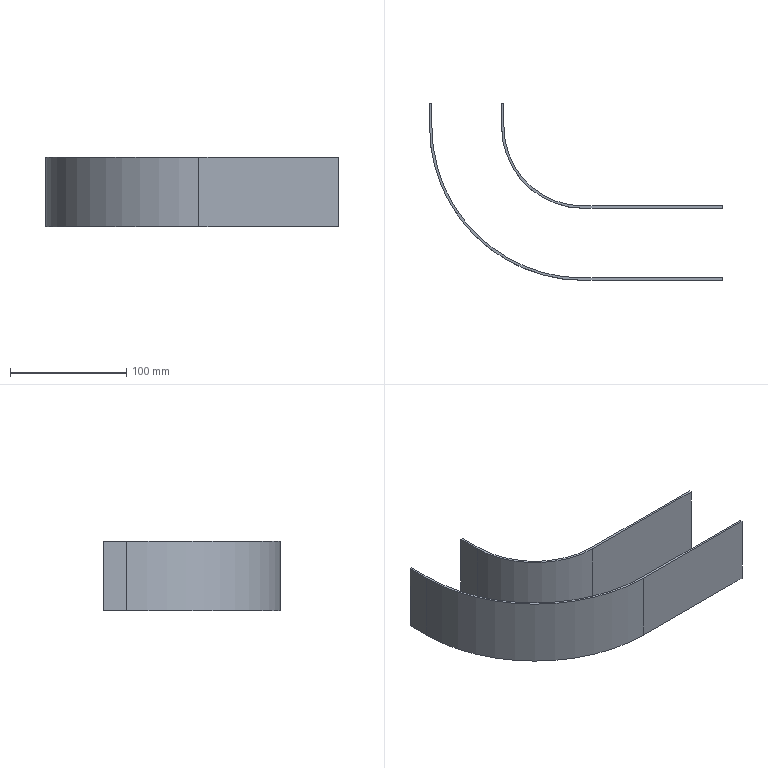Part | STEP file | 2 solids | 20 faces | box 252 x 152 x 60 mm | volume 71299 mm3 | plane 16 | cylinder 4 | commonest cylinder face diameters 136 x1 140 x1 260 x1 264 x1
STEP:
#1=CARTESIAN_POINT('',(0.,0.,0.));
#2=DIRECTION('',(0.,0.,1.));
#3=DIRECTION('',(1.,0.,0.));
#4=AXIS2_PLACEMENT_3D('',#1,#2,#3);
#5=CARTESIAN_POINT('',(100.,-32.,60.));
#6=VERTEX_POINT('',#5);
#7=CARTESIAN_POINT('',(-32.,100.,60.));
#8=VERTEX_POINT('',#7);
#9=CARTESIAN_POINT('',(100.,100.,60.));
#10=DIRECTION('',(0.,0.,-1.));
#11=DIRECTION('',(1.,0.,0.));
#12=AXIS2_PLACEMENT_3D('',#9,#10,#11);
#13=CIRCLE('',#12,132.);
#14=CARTESIAN_POINT('',(100.,100.,60.));
#15=DIRECTION('',(0.,0.,1.));
#16=DIRECTION('',(1.,0.,0.));
#17=AXIS2_PLACEMENT_3D('',#14,#15,#16);
#18=CYLINDRICAL_SURFACE('',#17,132.);
#19=CARTESIAN_POINT('',(6.283,0.));
#20=DIRECTION('',(-1.,0.));
#21=VECTOR('',#20,1.);
#22=LINE('',#19,#21);
#23=(GEOMETRIC_REPRESENTATION_CONTEXT(2)PARAMETRIC_REPRESENTATION_CONTEXT()REPRESENTATION_CONTEXT('',''));
#24=DEFINITIONAL_REPRESENTATION('',(#22),#23);
#25=PCURVE('',#18,#24);
#26=CARTESIAN_POINT('',(100.,100.,60.));
#27=DIRECTION('',(0.,0.,1.));
#28=DIRECTION('',(1.,0.,0.));
#29=AXIS2_PLACEMENT_3D('',#26,#27,#28);
#30=PLANE('',#29);
#31=CARTESIAN_POINT('',(132.,0.));
#32=CARTESIAN_POINT('',(132.,-228.631));
#33=CARTESIAN_POINT('',(-66.,-114.315));
#34=CARTESIAN_POINT('',(-264.,0.));
#35=CARTESIAN_POINT('',(-66.,114.315));
#36=CARTESIAN_POINT('',(132.,228.631));
#37=CARTESIAN_POINT('',(132.,0.));
#38=(BOUNDED_CURVE()B_SPLINE_CURVE(2,(#31,#32,#33,#34,#35,#36,#37),.UNSPECIFIED.,.T.,.F.)B_SPLINE_CURVE_WITH_KNOTS((1,2,2,2,2,1),(-2.094,0.,2.094,4.189,6.283,8.378),.UNSPECIFIED.)CURVE()GEOMETRIC_REPRESENTATION_ITEM()RATIONAL_B_SPLINE_CURVE((1.,0.5,1.,0.5,1.,0.5,1.))REPRESENTATION_ITEM(''));
#39=(GEOMETRIC_REPRESENTATION_CONTEXT(2)PARAMETRIC_REPRESENTATION_CONTEXT()REPRESENTATION_CONTEXT('',''));
#40=DEFINITIONAL_REPRESENTATION('',(#38),#39);
#41=PCURVE('',#30,#40);
#42=SURFACE_CURVE('',#13,(#25,#41),.PCURVE_S1.);
#43=EDGE_CURVE('',#6,#8,#42,.T.);
#44=ORIENTED_EDGE('',*,*,#43,.T.);
#45=CARTESIAN_POINT('',(-32.,100.,0.));
#46=VERTEX_POINT('',#45);
#47=CARTESIAN_POINT('',(-32.,100.,60.));
#48=DIRECTION('',(0.,0.,-1.));
#49=VECTOR('',#48,1.);
#50=LINE('',#47,#49);
#51=CARTESIAN_POINT('',(3.142,0.));
#52=DIRECTION('',(0.,-1.));
#53=VECTOR('',#52,1.);
#54=LINE('',#51,#53);
#55=(GEOMETRIC_REPRESENTATION_CONTEXT(2)PARAMETRIC_REPRESENTATION_CONTEXT()REPRESENTATION_CONTEXT('',''));
#56=DEFINITIONAL_REPRESENTATION('',(#54),#55);
#57=PCURVE('',#18,#56);
#58=CARTESIAN_POINT('',(-32.,100.,60.));
#59=DIRECTION('',(-1.,0.,0.));
#60=DIRECTION('',(0.,0.,1.));
#61=AXIS2_PLACEMENT_3D('',#58,#59,#60);
#62=PLANE('',#61);
#63=CARTESIAN_POINT('',(0.,0.));
#64=DIRECTION('',(-1.,0.));
#65=VECTOR('',#64,1.);
#66=LINE('',#63,#65);
#67=(GEOMETRIC_REPRESENTATION_CONTEXT(2)PARAMETRIC_REPRESENTATION_CONTEXT()REPRESENTATION_CONTEXT('',''));
#68=DEFINITIONAL_REPRESENTATION('',(#66),#67);
#69=PCURVE('',#62,#68);
#70=SURFACE_CURVE('',#50,(#57,#69),.PCURVE_S1.);
#71=EDGE_CURVE('',#8,#46,#70,.T.);
#72=ORIENTED_EDGE('',*,*,#71,.T.);
#73=CARTESIAN_POINT('',(100.,-32.,0.));
#74=VERTEX_POINT('',#73);
#75=CARTESIAN_POINT('',(100.,100.,0.));
#76=DIRECTION('',(0.,0.,1.));
#77=DIRECTION('',(1.,0.,0.));
#78=AXIS2_PLACEMENT_3D('',#75,#76,#77);
#79=CIRCLE('',#78,132.);
#80=CARTESIAN_POINT('',(0.,-60.));
#81=DIRECTION('',(1.,0.));
#82=VECTOR('',#81,1.);
#83=LINE('',#80,#82);
#84=(GEOMETRIC_REPRESENTATION_CONTEXT(2)PARAMETRIC_REPRESENTATION_CONTEXT()REPRESENTATION_CONTEXT('',''));
#85=DEFINITIONAL_REPRESENTATION('',(#83),#84);
#86=PCURVE('',#18,#85);
#87=CARTESIAN_POINT('',(100.,100.,0.));
#88=DIRECTION('',(0.,0.,1.));
#89=DIRECTION('',(1.,0.,0.));
#90=AXIS2_PLACEMENT_3D('',#87,#88,#89);
#91=PLANE('',#90);
#92=CARTESIAN_POINT('',(0.,0.));
#93=DIRECTION('',(1.,0.));
#94=AXIS2_PLACEMENT_2D('',#92,#93);
#95=CIRCLE('',#94,132.);
#96=(GEOMETRIC_REPRESENTATION_CONTEXT(2)PARAMETRIC_REPRESENTATION_CONTEXT()REPRESENTATION_CONTEXT('',''));
#97=DEFINITIONAL_REPRESENTATION('',(#95),#96);
#98=PCURVE('',#91,#97);
#99=SURFACE_CURVE('',#79,(#86,#98),.PCURVE_S1.);
#100=EDGE_CURVE('',#46,#74,#99,.T.);
#101=ORIENTED_EDGE('',*,*,#100,.T.);
#102=CARTESIAN_POINT('',(100.,-32.,60.));
#103=DIRECTION('',(0.,0.,1.));
#104=VECTOR('',#103,1.);
#105=LINE('',#102,#104);
#106=CARTESIAN_POINT('',(4.712,0.));
#107=DIRECTION('',(0.,1.));
#108=VECTOR('',#107,1.);
#109=LINE('',#106,#108);
#110=(GEOMETRIC_REPRESENTATION_CONTEXT(2)PARAMETRIC_REPRESENTATION_CONTEXT()REPRESENTATION_CONTEXT('',''));
#111=DEFINITIONAL_REPRESENTATION('',(#109),#110);
#112=PCURVE('',#18,#111);
#113=CARTESIAN_POINT('',(100.,-32.,60.));
#114=DIRECTION('',(0.,-1.,0.));
#115=DIRECTION('',(0.,0.,-1.));
#116=AXIS2_PLACEMENT_3D('',#113,#114,#115);
#117=PLANE('',#116);
#118=CARTESIAN_POINT('',(0.,0.));
#119=DIRECTION('',(-1.,0.));
#120=VECTOR('',#119,1.);
#121=LINE('',#118,#120);
#122=(GEOMETRIC_REPRESENTATION_CONTEXT(2)PARAMETRIC_REPRESENTATION_CONTEXT()REPRESENTATION_CONTEXT('',''));
#123=DEFINITIONAL_REPRESENTATION('',(#121),#122);
#124=PCURVE('',#117,#123);
#125=SURFACE_CURVE('',#105,(#112,#124),.PCURVE_S1.);
#126=EDGE_CURVE('',#74,#6,#125,.T.);
#127=ORIENTED_EDGE('',*,*,#126,.T.);
#128=EDGE_LOOP('',(#44,#72,#101,#127));
#129=FACE_BOUND('',#128,.T.);
#130=ADVANCED_FACE('',(#129),#18,.T.);
#131=CARTESIAN_POINT('',(-32.,120.,60.));
#132=VERTEX_POINT('',#131);
#133=CARTESIAN_POINT('',(-32.,100.,60.));
#134=DIRECTION('',(0.,1.,0.));
#135=VECTOR('',#134,1.);
#136=LINE('',#133,#135);
#137=CARTESIAN_POINT('',(0.,0.));
#138=DIRECTION('',(0.,1.));
#139=VECTOR('',#138,1.);
#140=LINE('',#137,#139);
#141=(GEOMETRIC_REPRESENTATION_CONTEXT(2)PARAMETRIC_REPRESENTATION_CONTEXT()REPRESENTATION_CONTEXT('',''));
#142=DEFINITIONAL_REPRESENTATION('',(#140),#141);
#143=PCURVE('',#62,#142);
#144=CARTESIAN_POINT('',(-132.,0.));
#145=DIRECTION('',(0.,1.));
#146=VECTOR('',#145,1.);
#147=LINE('',#144,#146);
#148=(GEOMETRIC_REPRESENTATION_CONTEXT(2)PARAMETRIC_REPRESENTATION_CONTEXT()REPRESENTATION_CONTEXT('',''));
#149=DEFINITIONAL_REPRESENTATION('',(#147),#148);
#150=PCURVE('',#30,#149);
#151=SURFACE_CURVE('',#136,(#143,#150),.PCURVE_S1.);
#152=EDGE_CURVE('',#8,#132,#151,.T.);
#153=ORIENTED_EDGE('',*,*,#152,.T.);
#154=CARTESIAN_POINT('',(-32.,120.,0.));
#155=VERTEX_POINT('',#154);
#156=CARTESIAN_POINT('',(-32.,120.,60.));
#157=DIRECTION('',(0.,0.,-1.));
#158=VECTOR('',#157,1.);
#159=LINE('',#156,#158);
#160=CARTESIAN_POINT('',(0.,20.));
#161=DIRECTION('',(-1.,0.));
#162=VECTOR('',#161,1.);
#163=LINE('',#160,#162);
#164=(GEOMETRIC_REPRESENTATION_CONTEXT(2)PARAMETRIC_REPRESENTATION_CONTEXT()REPRESENTATION_CONTEXT('',''));
#165=DEFINITIONAL_REPRESENTATION('',(#163),#164);
#166=PCURVE('',#62,#165);
#167=CARTESIAN_POINT('',(-32.,120.,60.));
#168=DIRECTION('',(0.,1.,0.));
#169=DIRECTION('',(0.,0.,1.));
#170=AXIS2_PLACEMENT_3D('',#167,#168,#169);
#171=PLANE('',#170);
#172=CARTESIAN_POINT('',(0.,0.));
#173=DIRECTION('',(-1.,0.));
#174=VECTOR('',#173,1.);
#175=LINE('',#172,#174);
#176=(GEOMETRIC_REPRESENTATION_CONTEXT(2)PARAMETRIC_REPRESENTATION_CONTEXT()REPRESENTATION_CONTEXT('',''));
#177=DEFINITIONAL_REPRESENTATION('',(#175),#176);
#178=PCURVE('',#171,#177);
#179=SURFACE_CURVE('',#159,(#166,#178),.PCURVE_S1.);
#180=EDGE_CURVE('',#132,#155,#179,.T.);
#181=ORIENTED_EDGE('',*,*,#180,.T.);
#182=CARTESIAN_POINT('',(-32.,100.,0.));
#183=DIRECTION('',(0.,-1.,0.));
#184=VECTOR('',#183,1.);
#185=LINE('',#182,#184);
#186=CARTESIAN_POINT('',(-60.,0.));
#187=DIRECTION('',(0.,-1.));
#188=VECTOR('',#187,1.);
#189=LINE('',#186,#188);
#190=(GEOMETRIC_REPRESENTATION_CONTEXT(2)PARAMETRIC_REPRESENTATION_CONTEXT()REPRESENTATION_CONTEXT('',''));
#191=DEFINITIONAL_REPRESENTATION('',(#189),#190);
#192=PCURVE('',#62,#191);
#193=CARTESIAN_POINT('',(-132.,0.));
#194=DIRECTION('',(0.,-1.));
#195=VECTOR('',#194,1.);
#196=LINE('',#193,#195);
#197=(GEOMETRIC_REPRESENTATION_CONTEXT(2)PARAMETRIC_REPRESENTATION_CONTEXT()REPRESENTATION_CONTEXT('',''));
#198=DEFINITIONAL_REPRESENTATION('',(#196),#197);
#199=PCURVE('',#91,#198);
#200=SURFACE_CURVE('',#185,(#192,#199),.PCURVE_S1.);
#201=EDGE_CURVE('',#155,#46,#200,.T.);
#202=ORIENTED_EDGE('',*,*,#201,.T.);
#203=ORIENTED_EDGE('',*,*,#71,.F.);
#204=EDGE_LOOP('',(#153,#181,#202,#203));
#205=FACE_BOUND('',#204,.T.);
#206=ADVANCED_FACE('',(#205),#62,.T.);
#207=CARTESIAN_POINT('',(220.,-32.,60.));
#208=VERTEX_POINT('',#207);
#209=CARTESIAN_POINT('',(220.,-30.,60.));
#210=VERTEX_POINT('',#209);
#211=CARTESIAN_POINT('',(220.,100.,60.));
#212=DIRECTION('',(0.,1.,0.));
#213=VECTOR('',#212,1.);
#214=LINE('',#211,#213);
#215=CARTESIAN_POINT('',(120.,0.));
#216=DIRECTION('',(0.,1.));
#217=VECTOR('',#216,1.);
#218=LINE('',#215,#217);
#219=(GEOMETRIC_REPRESENTATION_CONTEXT(2)PARAMETRIC_REPRESENTATION_CONTEXT()REPRESENTATION_CONTEXT('',''));
#220=DEFINITIONAL_REPRESENTATION('',(#218),#219);
#221=PCURVE('',#30,#220);
#222=CARTESIAN_POINT('',(220.,32.,60.));
#223=DIRECTION('',(1.,0.,0.));
#224=DIRECTION('',(0.,0.,-1.));
#225=AXIS2_PLACEMENT_3D('',#222,#223,#224);
#226=PLANE('',#225);
#227=CARTESIAN_POINT('',(0.,68.));
#228=DIRECTION('',(0.,1.));
#229=VECTOR('',#228,1.);
#230=LINE('',#227,#229);
#231=(GEOMETRIC_REPRESENTATION_CONTEXT(2)PARAMETRIC_REPRESENTATION_CONTEXT()REPRESENTATION_CONTEXT('',''));
#232=DEFINITIONAL_REPRESENTATION('',(#230),#231);
#233=PCURVE('',#226,#232);
#234=SURFACE_CURVE('',#214,(#221,#233),.PCURVE_S1.);
#235=EDGE_CURVE('',#208,#210,#234,.T.);
#236=ORIENTED_EDGE('',*,*,#235,.T.);
#237=CARTESIAN_POINT('',(100.,-30.,60.));
#238=VERTEX_POINT('',#237);
#239=CARTESIAN_POINT('',(100.,-30.,60.));
#240=DIRECTION('',(-1.,0.,0.));
#241=VECTOR('',#240,1.);
#242=LINE('',#239,#241);
#243=CARTESIAN_POINT('',(0.,-130.));
#244=DIRECTION('',(-1.,0.));
#245=VECTOR('',#244,1.);
#246=LINE('',#243,#245);
#247=(GEOMETRIC_REPRESENTATION_CONTEXT(2)PARAMETRIC_REPRESENTATION_CONTEXT()REPRESENTATION_CONTEXT('',''));
#248=DEFINITIONAL_REPRESENTATION('',(#246),#247);
#249=PCURVE('',#30,#248);
#250=CARTESIAN_POINT('',(100.,-30.,60.));
#251=DIRECTION('',(0.,-1.,0.));
#252=DIRECTION('',(0.,0.,-1.));
#253=AXIS2_PLACEMENT_3D('',#250,#251,#252);
#254=PLANE('',#253);
#255=CARTESIAN_POINT('',(0.,0.));
#256=DIRECTION('',(0.,-1.));
#257=VECTOR('',#256,1.);
#258=LINE('',#255,#257);
#259=(GEOMETRIC_REPRESENTATION_CONTEXT(2)PARAMETRIC_REPRESENTATION_CONTEXT()REPRESENTATION_CONTEXT('',''));
#260=DEFINITIONAL_REPRESENTATION('',(#258),#259);
#261=PCURVE('',#254,#260);
#262=SURFACE_CURVE('',#242,(#249,#261),.PCURVE_S1.);
#263=EDGE_CURVE('',#210,#238,#262,.T.);
#264=ORIENTED_EDGE('',*,*,#263,.T.);
#265=CARTESIAN_POINT('',(-30.,100.,60.));
#266=VERTEX_POINT('',#265);
#267=CARTESIAN_POINT('',(100.,100.,60.));
#268=DIRECTION('',(0.,0.,-1.));
#269=DIRECTION('',(1.,0.,0.));
#270=AXIS2_PLACEMENT_3D('',#267,#268,#269);
#271=CIRCLE('',#270,130.);
#272=CARTESIAN_POINT('',(130.,0.));
#273=CARTESIAN_POINT('',(130.,-225.167));
#274=CARTESIAN_POINT('',(-65.,-112.583));
#275=CARTESIAN_POINT('',(-260.,0.));
#276=CARTESIAN_POINT('',(-65.,112.583));
#277=CARTESIAN_POINT('',(130.,225.167));
#278=CARTESIAN_POINT('',(130.,0.));
#279=(BOUNDED_CURVE()B_SPLINE_CURVE(2,(#272,#273,#274,#275,#276,#277,#278),.UNSPECIFIED.,.T.,.F.)B_SPLINE_CURVE_WITH_KNOTS((1,2,2,2,2,1),(-2.094,0.,2.094,4.189,6.283,8.378),.UNSPECIFIED.)CURVE()GEOMETRIC_REPRESENTATION_ITEM()RATIONAL_B_SPLINE_CURVE((1.,0.5,1.,0.5,1.,0.5,1.))REPRESENTATION_ITEM(''));
#280=(GEOMETRIC_REPRESENTATION_CONTEXT(2)PARAMETRIC_REPRESENTATION_CONTEXT()REPRESENTATION_CONTEXT('',''));
#281=DEFINITIONAL_REPRESENTATION('',(#279),#280);
#282=PCURVE('',#30,#281);
#283=CARTESIAN_POINT('',(100.,100.,60.));
#284=DIRECTION('',(0.,0.,1.));
#285=DIRECTION('',(1.,0.,0.));
#286=AXIS2_PLACEMENT_3D('',#283,#284,#285);
#287=CYLINDRICAL_SURFACE('',#286,130.);
#288=CARTESIAN_POINT('',(6.283,0.));
#289=DIRECTION('',(-1.,0.));
#290=VECTOR('',#289,1.);
#291=LINE('',#288,#290);
#292=(GEOMETRIC_REPRESENTATION_CONTEXT(2)PARAMETRIC_REPRESENTATION_CONTEXT()REPRESENTATION_CONTEXT('',''));
#293=DEFINITIONAL_REPRESENTATION('',(#291),#292);
#294=PCURVE('',#287,#293);
#295=SURFACE_CURVE('',#271,(#282,#294),.PCURVE_S1.);
#296=EDGE_CURVE('',#238,#266,#295,.T.);
#297=ORIENTED_EDGE('',*,*,#296,.T.);
#298=CARTESIAN_POINT('',(-30.,120.,60.));
#299=VERTEX_POINT('',#298);
#300=CARTESIAN_POINT('',(-30.,100.,60.));
#301=DIRECTION('',(0.,1.,0.));
#302=VECTOR('',#301,1.);
#303=LINE('',#300,#302);
#304=CARTESIAN_POINT('',(-130.,0.));
#305=DIRECTION('',(0.,1.));
#306=VECTOR('',#305,1.);
#307=LINE('',#304,#306);
#308=(GEOMETRIC_REPRESENTATION_CONTEXT(2)PARAMETRIC_REPRESENTATION_CONTEXT()REPRESENTATION_CONTEXT('',''));
#309=DEFINITIONAL_REPRESENTATION('',(#307),#308);
#310=PCURVE('',#30,#309);
#311=CARTESIAN_POINT('',(-30.,100.,60.));
#312=DIRECTION('',(-1.,0.,0.));
#313=DIRECTION('',(0.,0.,1.));
#314=AXIS2_PLACEMENT_3D('',#311,#312,#313);
#315=PLANE('',#314);
#316=CARTESIAN_POINT('',(0.,0.));
#317=DIRECTION('',(0.,1.));
#318=VECTOR('',#317,1.);
#319=LINE('',#316,#318);
#320=(GEOMETRIC_REPRESENTATION_CONTEXT(2)PARAMETRIC_REPRESENTATION_CONTEXT()REPRESENTATION_CONTEXT('',''));
#321=DEFINITIONAL_REPRESENTATION('',(#319),#320);
#322=PCURVE('',#315,#321);
#323=SURFACE_CURVE('',#303,(#310,#322),.PCURVE_S1.);
#324=EDGE_CURVE('',#266,#299,#323,.T.);
#325=ORIENTED_EDGE('',*,*,#324,.T.);
#326=CARTESIAN_POINT('',(100.,120.,60.));
#327=DIRECTION('',(-1.,0.,0.));
#328=VECTOR('',#327,1.);
#329=LINE('',#326,#328);
#330=CARTESIAN_POINT('',(0.,20.));
#331=DIRECTION('',(-1.,0.));
#332=VECTOR('',#331,1.);
#333=LINE('',#330,#332);
#334=(GEOMETRIC_REPRESENTATION_CONTEXT(2)PARAMETRIC_REPRESENTATION_CONTEXT()REPRESENTATION_CONTEXT('',''));
#335=DEFINITIONAL_REPRESENTATION('',(#333),#334);
#336=PCURVE('',#30,#335);
#337=CARTESIAN_POINT('',(0.,132.));
#338=DIRECTION('',(0.,-1.));
#339=VECTOR('',#338,1.);
#340=LINE('',#337,#339);
#341=(GEOMETRIC_REPRESENTATION_CONTEXT(2)PARAMETRIC_REPRESENTATION_CONTEXT()REPRESENTATION_CONTEXT('',''));
#342=DEFINITIONAL_REPRESENTATION('',(#340),#341);
#343=PCURVE('',#171,#342);
#344=SURFACE_CURVE('',#329,(#336,#343),.PCURVE_S1.);
#345=EDGE_CURVE('',#299,#132,#344,.T.);
#346=ORIENTED_EDGE('',*,*,#345,.T.);
#347=ORIENTED_EDGE('',*,*,#152,.F.);
#348=ORIENTED_EDGE('',*,*,#43,.F.);
#349=CARTESIAN_POINT('',(100.,-32.,60.));
#350=DIRECTION('',(1.,0.,0.));
#351=VECTOR('',#350,1.);
#352=LINE('',#349,#351);
#353=CARTESIAN_POINT('',(0.,-132.));
#354=DIRECTION('',(1.,0.));
#355=VECTOR('',#354,1.);
#356=LINE('',#353,#355);
#357=(GEOMETRIC_REPRESENTATION_CONTEXT(2)PARAMETRIC_REPRESENTATION_CONTEXT()REPRESENTATION_CONTEXT('',''));
#358=DEFINITIONAL_REPRESENTATION('',(#356),#357);
#359=PCURVE('',#30,#358);
#360=CARTESIAN_POINT('',(0.,0.));
#361=DIRECTION('',(0.,1.));
#362=VECTOR('',#361,1.);
#363=LINE('',#360,#362);
#364=(GEOMETRIC_REPRESENTATION_CONTEXT(2)PARAMETRIC_REPRESENTATION_CONTEXT()REPRESENTATION_CONTEXT('',''));
#365=DEFINITIONAL_REPRESENTATION('',(#363),#364);
#366=PCURVE('',#117,#365);
#367=SURFACE_CURVE('',#352,(#359,#366),.PCURVE_S1.);
#368=EDGE_CURVE('',#6,#208,#367,.T.);
#369=ORIENTED_EDGE('',*,*,#368,.T.);
#370=EDGE_LOOP('',(#236,#264,#297,#325,#346,#347,#348,#369));
#371=FACE_BOUND('',#370,.T.);
#372=ADVANCED_FACE('',(#371),#30,.T.);
#373=ORIENTED_EDGE('',*,*,#368,.F.);
#374=ORIENTED_EDGE('',*,*,#126,.F.);
#375=CARTESIAN_POINT('',(220.,-32.,0.));
#376=VERTEX_POINT('',#375);
#377=CARTESIAN_POINT('',(100.,-32.,0.));
#378=DIRECTION('',(1.,0.,0.));
#379=VECTOR('',#378,1.);
#380=LINE('',#377,#379);
#381=CARTESIAN_POINT('',(60.,0.));
#382=DIRECTION('',(0.,1.));
#383=VECTOR('',#382,1.);
#384=LINE('',#381,#383);
#385=(GEOMETRIC_REPRESENTATION_CONTEXT(2)PARAMETRIC_REPRESENTATION_CONTEXT()REPRESENTATION_CONTEXT('',''));
#386=DEFINITIONAL_REPRESENTATION('',(#384),#385);
#387=PCURVE('',#117,#386);
#388=CARTESIAN_POINT('',(0.,-132.));
#389=DIRECTION('',(1.,0.));
#390=VECTOR('',#389,1.);
#391=LINE('',#388,#390);
#392=(GEOMETRIC_REPRESENTATION_CONTEXT(2)PARAMETRIC_REPRESENTATION_CONTEXT()REPRESENTATION_CONTEXT('',''));
#393=DEFINITIONAL_REPRESENTATION('',(#391),#392);
#394=PCURVE('',#91,#393);
#395=SURFACE_CURVE('',#380,(#387,#394),.PCURVE_S1.);
#396=EDGE_CURVE('',#74,#376,#395,.T.);
#397=ORIENTED_EDGE('',*,*,#396,.T.);
#398=CARTESIAN_POINT('',(220.,-32.,60.));
#399=DIRECTION('',(0.,0.,1.));
#400=VECTOR('',#399,1.);
#401=LINE('',#398,#400);
#402=CARTESIAN_POINT('',(0.,120.));
#403=DIRECTION('',(-1.,0.));
#404=VECTOR('',#403,1.);
#405=LINE('',#402,#404);
#406=(GEOMETRIC_REPRESENTATION_CONTEXT(2)PARAMETRIC_REPRESENTATION_CONTEXT()REPRESENTATION_CONTEXT('',''));
#407=DEFINITIONAL_REPRESENTATION('',(#405),#406);
#408=PCURVE('',#117,#407);
#409=CARTESIAN_POINT('',(0.,-64.));
#410=DIRECTION('',(-1.,0.));
#411=VECTOR('',#410,1.);
#412=LINE('',#409,#411);
#413=(GEOMETRIC_REPRESENTATION_CONTEXT(2)PARAMETRIC_REPRESENTATION_CONTEXT()REPRESENTATION_CONTEXT('',''));
#414=DEFINITIONAL_REPRESENTATION('',(#412),#413);
#415=PCURVE('',#226,#414);
#416=SURFACE_CURVE('',#401,(#408,#415),.PCURVE_S1.);
#417=EDGE_CURVE('',#376,#208,#416,.T.);
#418=ORIENTED_EDGE('',*,*,#417,.T.);
#419=EDGE_LOOP('',(#373,#374,#397,#418));
#420=FACE_BOUND('',#419,.T.);
#421=ADVANCED_FACE('',(#420),#117,.T.);
#422=CARTESIAN_POINT('',(220.,-30.,0.));
#423=VERTEX_POINT('',#422);
#424=CARTESIAN_POINT('',(100.,-30.,0.));
#425=VERTEX_POINT('',#424);
#426=CARTESIAN_POINT('',(100.,-30.,0.));
#427=DIRECTION('',(-1.,0.,0.));
#428=VECTOR('',#427,1.);
#429=LINE('',#426,#428);
#430=CARTESIAN_POINT('',(0.,-130.));
#431=DIRECTION('',(-1.,0.));
#432=VECTOR('',#431,1.);
#433=LINE('',#430,#432);
#434=(GEOMETRIC_REPRESENTATION_CONTEXT(2)PARAMETRIC_REPRESENTATION_CONTEXT()REPRESENTATION_CONTEXT('',''));
#435=DEFINITIONAL_REPRESENTATION('',(#433),#434);
#436=PCURVE('',#91,#435);
#437=CARTESIAN_POINT('',(60.,0.));
#438=DIRECTION('',(0.,-1.));
#439=VECTOR('',#438,1.);
#440=LINE('',#437,#439);
#441=(GEOMETRIC_REPRESENTATION_CONTEXT(2)PARAMETRIC_REPRESENTATION_CONTEXT()REPRESENTATION_CONTEXT('',''));
#442=DEFINITIONAL_REPRESENTATION('',(#440),#441);
#443=PCURVE('',#254,#442);
#444=SURFACE_CURVE('',#429,(#436,#443),.PCURVE_S1.);
#445=EDGE_CURVE('',#423,#425,#444,.T.);
#446=ORIENTED_EDGE('',*,*,#445,.F.);
#447=CARTESIAN_POINT('',(220.,100.,0.));
#448=DIRECTION('',(0.,1.,0.));
#449=VECTOR('',#448,1.);
#450=LINE('',#447,#449);
#451=CARTESIAN_POINT('',(120.,0.));
#452=DIRECTION('',(0.,1.));
#453=VECTOR('',#452,1.);
#454=LINE('',#451,#453);
#455=(GEOMETRIC_REPRESENTATION_CONTEXT(2)PARAMETRIC_REPRESENTATION_CONTEXT()REPRESENTATION_CONTEXT('',''));
#456=DEFINITIONAL_REPRESENTATION('',(#454),#455);
#457=PCURVE('',#91,#456);
#458=CARTESIAN_POINT('',(60.,68.));
#459=DIRECTION('',(0.,1.));
#460=VECTOR('',#459,1.);
#461=LINE('',#458,#460);
#462=(GEOMETRIC_REPRESENTATION_CONTEXT(2)PARAMETRIC_REPRESENTATION_CONTEXT()REPRESENTATION_CONTEXT('',''));
#463=DEFINITIONAL_REPRESENTATION('',(#461),#462);
#464=PCURVE('',#226,#463);
#465=SURFACE_CURVE('',#450,(#457,#464),.PCURVE_S1.);
#466=EDGE_CURVE('',#376,#423,#465,.T.);
#467=ORIENTED_EDGE('',*,*,#466,.F.);
#468=ORIENTED_EDGE('',*,*,#396,.F.);
#469=ORIENTED_EDGE('',*,*,#100,.F.);
#470=ORIENTED_EDGE('',*,*,#201,.F.);
#471=CARTESIAN_POINT('',(-30.,120.,0.));
#472=VERTEX_POINT('',#471);
#473=CARTESIAN_POINT('',(100.,120.,0.));
#474=DIRECTION('',(-1.,0.,0.));
#475=VECTOR('',#474,1.);
#476=LINE('',#473,#475);
#477=CARTESIAN_POINT('',(0.,20.));
#478=DIRECTION('',(-1.,0.));
#479=VECTOR('',#478,1.);
#480=LINE('',#477,#479);
#481=(GEOMETRIC_REPRESENTATION_CONTEXT(2)PARAMETRIC_REPRESENTATION_CONTEXT()REPRESENTATION_CONTEXT('',''));
#482=DEFINITIONAL_REPRESENTATION('',(#480),#481);
#483=PCURVE('',#91,#482);
#484=CARTESIAN_POINT('',(-60.,132.));
#485=DIRECTION('',(0.,-1.));
#486=VECTOR('',#485,1.);
#487=LINE('',#484,#486);
#488=(GEOMETRIC_REPRESENTATION_CONTEXT(2)PARAMETRIC_REPRESENTATION_CONTEXT()REPRESENTATION_CONTEXT('',''));
#489=DEFINITIONAL_REPRESENTATION('',(#487),#488);
#490=PCURVE('',#171,#489);
#491=SURFACE_CURVE('',#476,(#483,#490),.PCURVE_S1.);
#492=EDGE_CURVE('',#472,#155,#491,.T.);
#493=ORIENTED_EDGE('',*,*,#492,.F.);
#494=CARTESIAN_POINT('',(-30.,100.,0.));
#495=VERTEX_POINT('',#494);
#496=CARTESIAN_POINT('',(-30.,100.,0.));
#497=DIRECTION('',(0.,1.,0.));
#498=VECTOR('',#497,1.);
#499=LINE('',#496,#498);
#500=CARTESIAN_POINT('',(-130.,0.));
#501=DIRECTION('',(0.,1.));
#502=VECTOR('',#501,1.);
#503=LINE('',#500,#502);
#504=(GEOMETRIC_REPRESENTATION_CONTEXT(2)PARAMETRIC_REPRESENTATION_CONTEXT()REPRESENTATION_CONTEXT('',''));
#505=DEFINITIONAL_REPRESENTATION('',(#503),#504);
#506=PCURVE('',#91,#505);
#507=CARTESIAN_POINT('',(-60.,0.));
#508=DIRECTION('',(0.,1.));
#509=VECTOR('',#508,1.);
#510=LINE('',#507,#509);
#511=(GEOMETRIC_REPRESENTATION_CONTEXT(2)PARAMETRIC_REPRESENTATION_CONTEXT()REPRESENTATION_CONTEXT('',''));
#512=DEFINITIONAL_REPRESENTATION('',(#510),#511);
#513=PCURVE('',#315,#512);
#514=SURFACE_CURVE('',#499,(#506,#513),.PCURVE_S1.);
#515=EDGE_CURVE('',#495,#472,#514,.T.);
#516=ORIENTED_EDGE('',*,*,#515,.F.);
#517=CARTESIAN_POINT('',(100.,100.,0.));
#518=DIRECTION('',(0.,0.,-1.));
#519=DIRECTION('',(1.,0.,0.));
#520=AXIS2_PLACEMENT_3D('',#517,#518,#519);
#521=CIRCLE('',#520,130.);
#522=CARTESIAN_POINT('',(130.,0.));
#523=CARTESIAN_POINT('',(130.,-225.167));
#524=CARTESIAN_POINT('',(-65.,-112.583));
#525=CARTESIAN_POINT('',(-260.,0.));
#526=CARTESIAN_POINT('',(-65.,112.583));
#527=CARTESIAN_POINT('',(130.,225.167));
#528=CARTESIAN_POINT('',(130.,0.));
#529=(BOUNDED_CURVE()B_SPLINE_CURVE(2,(#522,#523,#524,#525,#526,#527,#528),.UNSPECIFIED.,.T.,.F.)B_SPLINE_CURVE_WITH_KNOTS((1,2,2,2,2,1),(-2.094,0.,2.094,4.189,6.283,8.378),.UNSPECIFIED.)CURVE()GEOMETRIC_REPRESENTATION_ITEM()RATIONAL_B_SPLINE_CURVE((1.,0.5,1.,0.5,1.,0.5,1.))REPRESENTATION_ITEM(''));
#530=(GEOMETRIC_REPRESENTATION_CONTEXT(2)PARAMETRIC_REPRESENTATION_CONTEXT()REPRESENTATION_CONTEXT('',''));
#531=DEFINITIONAL_REPRESENTATION('',(#529),#530);
#532=PCURVE('',#91,#531);
#533=CARTESIAN_POINT('',(6.283,-60.));
#534=DIRECTION('',(-1.,0.));
#535=VECTOR('',#534,1.);
#536=LINE('',#533,#535);
#537=(GEOMETRIC_REPRESENTATION_CONTEXT(2)PARAMETRIC_REPRESENTATION_CONTEXT()REPRESENTATION_CONTEXT('',''));
#538=DEFINITIONAL_REPRESENTATION('',(#536),#537);
#539=PCURVE('',#287,#538);
#540=SURFACE_CURVE('',#521,(#532,#539),.PCURVE_S1.);
#541=EDGE_CURVE('',#425,#495,#540,.T.);
#542=ORIENTED_EDGE('',*,*,#541,.F.);
#543=EDGE_LOOP('',(#446,#467,#468,#469,#470,#493,#516,#542));
#544=FACE_BOUND('',#543,.T.);
#545=ADVANCED_FACE('',(#544),#91,.F.);
#546=ORIENTED_EDGE('',*,*,#180,.F.);
#547=ORIENTED_EDGE('',*,*,#345,.F.);
#548=CARTESIAN_POINT('',(-30.,120.,60.));
#549=DIRECTION('',(0.,0.,-1.));
#550=VECTOR('',#549,1.);
#551=LINE('',#548,#550);
#552=CARTESIAN_POINT('',(0.,2.));
#553=DIRECTION('',(-1.,0.));
#554=VECTOR('',#553,1.);
#555=LINE('',#552,#554);
#556=(GEOMETRIC_REPRESENTATION_CONTEXT(2)PARAMETRIC_REPRESENTATION_CONTEXT()REPRESENTATION_CONTEXT('',''));
#557=DEFINITIONAL_REPRESENTATION('',(#555),#556);
#558=PCURVE('',#171,#557);
#559=CARTESIAN_POINT('',(0.,20.));
#560=DIRECTION('',(-1.,0.));
#561=VECTOR('',#560,1.);
#562=LINE('',#559,#561);
#563=(GEOMETRIC_REPRESENTATION_CONTEXT(2)PARAMETRIC_REPRESENTATION_CONTEXT()REPRESENTATION_CONTEXT('',''));
#564=DEFINITIONAL_REPRESENTATION('',(#562),#563);
#565=PCURVE('',#315,#564);
#566=SURFACE_CURVE('',#551,(#558,#565),.PCURVE_S1.);
#567=EDGE_CURVE('',#299,#472,#566,.T.);
#568=ORIENTED_EDGE('',*,*,#567,.T.);
#569=ORIENTED_EDGE('',*,*,#492,.T.);
#570=EDGE_LOOP('',(#546,#547,#568,#569));
#571=FACE_BOUND('',#570,.T.);
#572=ADVANCED_FACE('',(#571),#171,.T.);
#573=CARTESIAN_POINT('',(220.,-30.,60.));
#574=DIRECTION('',(0.,0.,1.));
#575=VECTOR('',#574,1.);
#576=LINE('',#573,#575);
#577=CARTESIAN_POINT('',(0.,120.));
#578=DIRECTION('',(-1.,0.));
#579=VECTOR('',#578,1.);
#580=LINE('',#577,#579);
#581=(GEOMETRIC_REPRESENTATION_CONTEXT(2)PARAMETRIC_REPRESENTATION_CONTEXT()REPRESENTATION_CONTEXT('',''));
#582=DEFINITIONAL_REPRESENTATION('',(#580),#581);
#583=PCURVE('',#254,#582);
#584=CARTESIAN_POINT('',(0.,-62.));
#585=DIRECTION('',(-1.,0.));
#586=VECTOR('',#585,1.);
#587=LINE('',#584,#586);
#588=(GEOMETRIC_REPRESENTATION_CONTEXT(2)PARAMETRIC_REPRESENTATION_CONTEXT()REPRESENTATION_CONTEXT('',''));
#589=DEFINITIONAL_REPRESENTATION('',(#587),#588);
#590=PCURVE('',#226,#589);
#591=SURFACE_CURVE('',#576,(#583,#590),.PCURVE_S1.);
#592=EDGE_CURVE('',#423,#210,#591,.T.);
#593=ORIENTED_EDGE('',*,*,#592,.F.);
#594=ORIENTED_EDGE('',*,*,#445,.T.);
#595=CARTESIAN_POINT('',(100.,-30.,60.));
#596=DIRECTION('',(0.,0.,-1.));
#597=VECTOR('',#596,1.);
#598=LINE('',#595,#597);
#599=CARTESIAN_POINT('',(0.,0.));
#600=DIRECTION('',(1.,0.));
#601=VECTOR('',#600,1.);
#602=LINE('',#599,#601);
#603=(GEOMETRIC_REPRESENTATION_CONTEXT(2)PARAMETRIC_REPRESENTATION_CONTEXT()REPRESENTATION_CONTEXT('',''));
#604=DEFINITIONAL_REPRESENTATION('',(#602),#603);
#605=PCURVE('',#254,#604);
#606=CARTESIAN_POINT('',(4.712,0.));
#607=DIRECTION('',(0.,-1.));
#608=VECTOR('',#607,1.);
#609=LINE('',#606,#608);
#610=(GEOMETRIC_REPRESENTATION_CONTEXT(2)PARAMETRIC_REPRESENTATION_CONTEXT()REPRESENTATION_CONTEXT('',''));
#611=DEFINITIONAL_REPRESENTATION('',(#609),#610);
#612=PCURVE('',#287,#611);
#613=SURFACE_CURVE('',#598,(#605,#612),.PCURVE_S1.);
#614=EDGE_CURVE('',#238,#425,#613,.T.);
#615=ORIENTED_EDGE('',*,*,#614,.F.);
#616=ORIENTED_EDGE('',*,*,#263,.F.);
#617=EDGE_LOOP('',(#593,#594,#615,#616));
#618=FACE_BOUND('',#617,.T.);
#619=ADVANCED_FACE('',(#618),#254,.F.);
#620=ORIENTED_EDGE('',*,*,#417,.F.);
#621=ORIENTED_EDGE('',*,*,#466,.T.);
#622=ORIENTED_EDGE('',*,*,#592,.T.);
#623=ORIENTED_EDGE('',*,*,#235,.F.);
#624=EDGE_LOOP('',(#620,#621,#622,#623));
#625=FACE_BOUND('',#624,.T.);
#626=ADVANCED_FACE('',(#625),#226,.T.);
#627=ORIENTED_EDGE('',*,*,#515,.T.);
#628=ORIENTED_EDGE('',*,*,#567,.F.);
#629=ORIENTED_EDGE('',*,*,#324,.F.);
#630=CARTESIAN_POINT('',(-30.,100.,60.));
#631=DIRECTION('',(0.,0.,1.));
#632=VECTOR('',#631,1.);
#633=LINE('',#630,#632);
#634=CARTESIAN_POINT('',(0.,0.));
#635=DIRECTION('',(1.,0.));
#636=VECTOR('',#635,1.);
#637=LINE('',#634,#636);
#638=(GEOMETRIC_REPRESENTATION_CONTEXT(2)PARAMETRIC_REPRESENTATION_CONTEXT()REPRESENTATION_CONTEXT('',''));
#639=DEFINITIONAL_REPRESENTATION('',(#637),#638);
#640=PCURVE('',#315,#639);
#641=CARTESIAN_POINT('',(3.142,0.));
#642=DIRECTION('',(0.,1.));
#643=VECTOR('',#642,1.);
#644=LINE('',#641,#643);
#645=(GEOMETRIC_REPRESENTATION_CONTEXT(2)PARAMETRIC_REPRESENTATION_CONTEXT()REPRESENTATION_CONTEXT('',''));
#646=DEFINITIONAL_REPRESENTATION('',(#644),#645);
#647=PCURVE('',#287,#646);
#648=SURFACE_CURVE('',#633,(#640,#647),.PCURVE_S1.);
#649=EDGE_CURVE('',#495,#266,#648,.T.);
#650=ORIENTED_EDGE('',*,*,#649,.F.);
#651=EDGE_LOOP('',(#627,#628,#629,#650));
#652=FACE_BOUND('',#651,.T.);
#653=ADVANCED_FACE('',(#652),#315,.F.);
#654=ORIENTED_EDGE('',*,*,#614,.F.);
#655=ORIENTED_EDGE('',*,*,#296,.T.);
#656=ORIENTED_EDGE('',*,*,#649,.F.);
#657=ORIENTED_EDGE('',*,*,#541,.F.);
#658=EDGE_LOOP('',(#654,#655,#656,#657));
#659=FACE_BOUND('',#658,.F.);
#660=ADVANCED_FACE('',(#659),#287,.F.);
#661=CLOSED_SHELL('',(#130,#206,#372,#421,#545,#572,#619,#626,#653,#660));
#662=MANIFOLD_SOLID_BREP('',#661);
#663=CARTESIAN_POINT('',(100.,32.,60.));
#664=VERTEX_POINT('',#663);
#665=CARTESIAN_POINT('',(100.,32.,0.));
#666=VERTEX_POINT('',#665);
#667=CARTESIAN_POINT('',(100.,32.,60.));
#668=DIRECTION('',(0.,0.,-1.));
#669=VECTOR('',#668,1.);
#670=LINE('',#667,#669);
#671=CARTESIAN_POINT('',(100.,32.,60.));
#672=DIRECTION('',(0.,-1.,0.));
#673=DIRECTION('',(0.,0.,-1.));
#674=AXIS2_PLACEMENT_3D('',#671,#672,#673);
#675=PLANE('',#674);
#676=CARTESIAN_POINT('',(0.,0.));
#677=DIRECTION('',(1.,0.));
#678=VECTOR('',#677,1.);
#679=LINE('',#676,#678);
#680=(GEOMETRIC_REPRESENTATION_CONTEXT(2)PARAMETRIC_REPRESENTATION_CONTEXT()REPRESENTATION_CONTEXT('',''));
#681=DEFINITIONAL_REPRESENTATION('',(#679),#680);
#682=PCURVE('',#675,#681);
#683=CARTESIAN_POINT('',(100.,100.,60.));
#684=DIRECTION('',(0.,0.,1.));
#685=DIRECTION('',(1.,0.,0.));
#686=AXIS2_PLACEMENT_3D('',#683,#684,#685);
#687=CYLINDRICAL_SURFACE('',#686,68.);
#688=CARTESIAN_POINT('',(4.712,0.));
#689=DIRECTION('',(0.,-1.));
#690=VECTOR('',#689,1.);
#691=LINE('',#688,#690);
#692=(GEOMETRIC_REPRESENTATION_CONTEXT(2)PARAMETRIC_REPRESENTATION_CONTEXT()REPRESENTATION_CONTEXT('',''));
#693=DEFINITIONAL_REPRESENTATION('',(#691),#692);
#694=PCURVE('',#687,#693);
#695=SURFACE_CURVE('',#670,(#682,#694),.PCURVE_S1.);
#696=EDGE_CURVE('',#664,#666,#695,.T.);
#697=ORIENTED_EDGE('',*,*,#696,.F.);
#698=CARTESIAN_POINT('',(220.,32.,60.));
#699=VERTEX_POINT('',#698);
#700=CARTESIAN_POINT('',(100.,32.,60.));
#701=DIRECTION('',(-1.,0.,0.));
#702=VECTOR('',#701,1.);
#703=LINE('',#700,#702);
#704=CARTESIAN_POINT('',(0.,0.));
#705=DIRECTION('',(0.,-1.));
#706=VECTOR('',#705,1.);
#707=LINE('',#704,#706);
#708=(GEOMETRIC_REPRESENTATION_CONTEXT(2)PARAMETRIC_REPRESENTATION_CONTEXT()REPRESENTATION_CONTEXT('',''));
#709=DEFINITIONAL_REPRESENTATION('',(#707),#708);
#710=PCURVE('',#675,#709);
#711=CARTESIAN_POINT('',(100.,100.,60.));
#712=DIRECTION('',(0.,0.,1.));
#713=DIRECTION('',(1.,0.,0.));
#714=AXIS2_PLACEMENT_3D('',#711,#712,#713);
#715=PLANE('',#714);
#716=CARTESIAN_POINT('',(0.,-68.));
#717=DIRECTION('',(-1.,0.));
#718=VECTOR('',#717,1.);
#719=LINE('',#716,#718);
#720=(GEOMETRIC_REPRESENTATION_CONTEXT(2)PARAMETRIC_REPRESENTATION_CONTEXT()REPRESENTATION_CONTEXT('',''));
#721=DEFINITIONAL_REPRESENTATION('',(#719),#720);
#722=PCURVE('',#715,#721);
#723=SURFACE_CURVE('',#703,(#710,#722),.PCURVE_S1.);
#724=EDGE_CURVE('',#699,#664,#723,.T.);
#725=ORIENTED_EDGE('',*,*,#724,.F.);
#726=CARTESIAN_POINT('',(220.,32.,0.));
#727=VERTEX_POINT('',#726);
#728=CARTESIAN_POINT('',(220.,32.,60.));
#729=DIRECTION('',(0.,0.,1.));
#730=VECTOR('',#729,1.);
#731=LINE('',#728,#730);
#732=CARTESIAN_POINT('',(0.,120.));
#733=DIRECTION('',(-1.,0.));
#734=VECTOR('',#733,1.);
#735=LINE('',#732,#734);
#736=(GEOMETRIC_REPRESENTATION_CONTEXT(2)PARAMETRIC_REPRESENTATION_CONTEXT()REPRESENTATION_CONTEXT('',''));
#737=DEFINITIONAL_REPRESENTATION('',(#735),#736);
#738=PCURVE('',#675,#737);
#739=CARTESIAN_POINT('',(220.,32.,60.));
#740=DIRECTION('',(1.,0.,0.));
#741=DIRECTION('',(0.,0.,-1.));
#742=AXIS2_PLACEMENT_3D('',#739,#740,#741);
#743=PLANE('',#742);
#744=CARTESIAN_POINT('',(0.,0.));
#745=DIRECTION('',(-1.,0.));
#746=VECTOR('',#745,1.);
#747=LINE('',#744,#746);
#748=(GEOMETRIC_REPRESENTATION_CONTEXT(2)PARAMETRIC_REPRESENTATION_CONTEXT()REPRESENTATION_CONTEXT('',''));
#749=DEFINITIONAL_REPRESENTATION('',(#747),#748);
#750=PCURVE('',#743,#749);
#751=SURFACE_CURVE('',#731,(#738,#750),.PCURVE_S1.);
#752=EDGE_CURVE('',#727,#699,#751,.T.);
#753=ORIENTED_EDGE('',*,*,#752,.F.);
#754=CARTESIAN_POINT('',(100.,32.,0.));
#755=DIRECTION('',(1.,0.,0.));
#756=VECTOR('',#755,1.);
#757=LINE('',#754,#756);
#758=CARTESIAN_POINT('',(60.,0.));
#759=DIRECTION('',(0.,1.));
#760=VECTOR('',#759,1.);
#761=LINE('',#758,#760);
#762=(GEOMETRIC_REPRESENTATION_CONTEXT(2)PARAMETRIC_REPRESENTATION_CONTEXT()REPRESENTATION_CONTEXT('',''));
#763=DEFINITIONAL_REPRESENTATION('',(#761),#762);
#764=PCURVE('',#675,#763);
#765=CARTESIAN_POINT('',(100.,100.,0.));
#766=DIRECTION('',(0.,0.,1.));
#767=DIRECTION('',(1.,0.,0.));
#768=AXIS2_PLACEMENT_3D('',#765,#766,#767);
#769=PLANE('',#768);
#770=CARTESIAN_POINT('',(0.,-68.));
#771=DIRECTION('',(1.,0.));
#772=VECTOR('',#771,1.);
#773=LINE('',#770,#772);
#774=(GEOMETRIC_REPRESENTATION_CONTEXT(2)PARAMETRIC_REPRESENTATION_CONTEXT()REPRESENTATION_CONTEXT('',''));
#775=DEFINITIONAL_REPRESENTATION('',(#773),#774);
#776=PCURVE('',#769,#775);
#777=SURFACE_CURVE('',#757,(#764,#776),.PCURVE_S1.);
#778=EDGE_CURVE('',#666,#727,#777,.T.);
#779=ORIENTED_EDGE('',*,*,#778,.F.);
#780=EDGE_LOOP('',(#697,#725,#753,#779));
#781=FACE_BOUND('',#780,.T.);
#782=ADVANCED_FACE('',(#781),#675,.F.);
#783=CARTESIAN_POINT('',(100.,30.,0.));
#784=VERTEX_POINT('',#783);
#785=CARTESIAN_POINT('',(220.,30.,0.));
#786=VERTEX_POINT('',#785);
#787=CARTESIAN_POINT('',(100.,30.,0.));
#788=DIRECTION('',(1.,0.,0.));
#789=VECTOR('',#788,1.);
#790=LINE('',#787,#789);
#791=CARTESIAN_POINT('',(0.,-70.));
#792=DIRECTION('',(1.,0.));
#793=VECTOR('',#792,1.);
#794=LINE('',#791,#793);
#795=(GEOMETRIC_REPRESENTATION_CONTEXT(2)PARAMETRIC_REPRESENTATION_CONTEXT()REPRESENTATION_CONTEXT('',''));
#796=DEFINITIONAL_REPRESENTATION('',(#794),#795);
#797=PCURVE('',#769,#796);
#798=CARTESIAN_POINT('',(100.,30.,60.));
#799=DIRECTION('',(0.,-1.,0.));
#800=DIRECTION('',(0.,0.,-1.));
#801=AXIS2_PLACEMENT_3D('',#798,#799,#800);
#802=PLANE('',#801);
#803=CARTESIAN_POINT('',(60.,0.));
#804=DIRECTION('',(0.,1.));
#805=VECTOR('',#804,1.);
#806=LINE('',#803,#805);
#807=(GEOMETRIC_REPRESENTATION_CONTEXT(2)PARAMETRIC_REPRESENTATION_CONTEXT()REPRESENTATION_CONTEXT('',''));
#808=DEFINITIONAL_REPRESENTATION('',(#806),#807);
#809=PCURVE('',#802,#808);
#810=SURFACE_CURVE('',#790,(#797,#809),.PCURVE_S1.);
#811=EDGE_CURVE('',#784,#786,#810,.T.);
#812=ORIENTED_EDGE('',*,*,#811,.F.);
#813=CARTESIAN_POINT('',(30.,100.,0.));
#814=VERTEX_POINT('',#813);
#815=CARTESIAN_POINT('',(100.,100.,0.));
#816=DIRECTION('',(0.,0.,1.));
#817=DIRECTION('',(1.,0.,0.));
#818=AXIS2_PLACEMENT_3D('',#815,#816,#817);
#819=CIRCLE('',#818,70.);
#820=CARTESIAN_POINT('',(0.,0.));
#821=DIRECTION('',(1.,0.));
#822=AXIS2_PLACEMENT_2D('',#820,#821);
#823=CIRCLE('',#822,70.);
#824=(GEOMETRIC_REPRESENTATION_CONTEXT(2)PARAMETRIC_REPRESENTATION_CONTEXT()REPRESENTATION_CONTEXT('',''));
#825=DEFINITIONAL_REPRESENTATION('',(#823),#824);
#826=PCURVE('',#769,#825);
#827=CARTESIAN_POINT('',(100.,100.,60.));
#828=DIRECTION('',(0.,0.,1.));
#829=DIRECTION('',(1.,0.,0.));
#830=AXIS2_PLACEMENT_3D('',#827,#828,#829);
#831=CYLINDRICAL_SURFACE('',#830,70.);
#832=CARTESIAN_POINT('',(0.,-60.));
#833=DIRECTION('',(1.,0.));
#834=VECTOR('',#833,1.);
#835=LINE('',#832,#834);
#836=(GEOMETRIC_REPRESENTATION_CONTEXT(2)PARAMETRIC_REPRESENTATION_CONTEXT()REPRESENTATION_CONTEXT('',''));
#837=DEFINITIONAL_REPRESENTATION('',(#835),#836);
#838=PCURVE('',#831,#837);
#839=SURFACE_CURVE('',#819,(#826,#838),.PCURVE_S1.);
#840=EDGE_CURVE('',#814,#784,#839,.T.);
#841=ORIENTED_EDGE('',*,*,#840,.F.);
#842=CARTESIAN_POINT('',(30.,120.,0.));
#843=VERTEX_POINT('',#842);
#844=CARTESIAN_POINT('',(30.,100.,0.));
#845=DIRECTION('',(0.,-1.,0.));
#846=VECTOR('',#845,1.);
#847=LINE('',#844,#846);
#848=CARTESIAN_POINT('',(-70.,0.));
#849=DIRECTION('',(0.,-1.));
#850=VECTOR('',#849,1.);
#851=LINE('',#848,#850);
#852=(GEOMETRIC_REPRESENTATION_CONTEXT(2)PARAMETRIC_REPRESENTATION_CONTEXT()REPRESENTATION_CONTEXT('',''));
#853=DEFINITIONAL_REPRESENTATION('',(#851),#852);
#854=PCURVE('',#769,#853);
#855=CARTESIAN_POINT('',(30.,100.,60.));
#856=DIRECTION('',(-1.,0.,0.));
#857=DIRECTION('',(0.,0.,1.));
#858=AXIS2_PLACEMENT_3D('',#855,#856,#857);
#859=PLANE('',#858);
#860=CARTESIAN_POINT('',(-60.,0.));
#861=DIRECTION('',(0.,-1.));
#862=VECTOR('',#861,1.);
#863=LINE('',#860,#862);
#864=(GEOMETRIC_REPRESENTATION_CONTEXT(2)PARAMETRIC_REPRESENTATION_CONTEXT()REPRESENTATION_CONTEXT('',''));
#865=DEFINITIONAL_REPRESENTATION('',(#863),#864);
#866=PCURVE('',#859,#865);
#867=SURFACE_CURVE('',#847,(#854,#866),.PCURVE_S1.);
#868=EDGE_CURVE('',#843,#814,#867,.T.);
#869=ORIENTED_EDGE('',*,*,#868,.F.);
#870=CARTESIAN_POINT('',(32.,120.,0.));
#871=VERTEX_POINT('',#870);
#872=CARTESIAN_POINT('',(100.,120.,0.));
#873=DIRECTION('',(-1.,0.,0.));
#874=VECTOR('',#873,1.);
#875=LINE('',#872,#874);
#876=CARTESIAN_POINT('',(0.,20.));
#877=DIRECTION('',(-1.,0.));
#878=VECTOR('',#877,1.);
#879=LINE('',#876,#878);
#880=(GEOMETRIC_REPRESENTATION_CONTEXT(2)PARAMETRIC_REPRESENTATION_CONTEXT()REPRESENTATION_CONTEXT('',''));
#881=DEFINITIONAL_REPRESENTATION('',(#879),#880);
#882=PCURVE('',#769,#881);
#883=CARTESIAN_POINT('',(-32.,120.,60.));
#884=DIRECTION('',(0.,1.,0.));
#885=DIRECTION('',(0.,0.,1.));
#886=AXIS2_PLACEMENT_3D('',#883,#884,#885);
#887=PLANE('',#886);
#888=CARTESIAN_POINT('',(-60.,132.));
#889=DIRECTION('',(0.,-1.));
#890=VECTOR('',#889,1.);
#891=LINE('',#888,#890);
#892=(GEOMETRIC_REPRESENTATION_CONTEXT(2)PARAMETRIC_REPRESENTATION_CONTEXT()REPRESENTATION_CONTEXT('',''));
#893=DEFINITIONAL_REPRESENTATION('',(#891),#892);
#894=PCURVE('',#887,#893);
#895=SURFACE_CURVE('',#875,(#882,#894),.PCURVE_S1.);
#896=EDGE_CURVE('',#871,#843,#895,.T.);
#897=ORIENTED_EDGE('',*,*,#896,.F.);
#898=CARTESIAN_POINT('',(32.,100.,0.));
#899=VERTEX_POINT('',#898);
#900=CARTESIAN_POINT('',(32.,100.,0.));
#901=DIRECTION('',(0.,1.,0.));
#902=VECTOR('',#901,1.);
#903=LINE('',#900,#902);
#904=CARTESIAN_POINT('',(-68.,0.));
#905=DIRECTION('',(0.,1.));
#906=VECTOR('',#905,1.);
#907=LINE('',#904,#906);
#908=(GEOMETRIC_REPRESENTATION_CONTEXT(2)PARAMETRIC_REPRESENTATION_CONTEXT()REPRESENTATION_CONTEXT('',''));
#909=DEFINITIONAL_REPRESENTATION('',(#907),#908);
#910=PCURVE('',#769,#909);
#911=CARTESIAN_POINT('',(32.,100.,60.));
#912=DIRECTION('',(-1.,0.,0.));
#913=DIRECTION('',(0.,0.,1.));
#914=AXIS2_PLACEMENT_3D('',#911,#912,#913);
#915=PLANE('',#914);
#916=CARTESIAN_POINT('',(-60.,0.));
#917=DIRECTION('',(0.,1.));
#918=VECTOR('',#917,1.);
#919=LINE('',#916,#918);
#920=(GEOMETRIC_REPRESENTATION_CONTEXT(2)PARAMETRIC_REPRESENTATION_CONTEXT()REPRESENTATION_CONTEXT('',''));
#921=DEFINITIONAL_REPRESENTATION('',(#919),#920);
#922=PCURVE('',#915,#921);
#923=SURFACE_CURVE('',#903,(#910,#922),.PCURVE_S1.);
#924=EDGE_CURVE('',#899,#871,#923,.T.);
#925=ORIENTED_EDGE('',*,*,#924,.F.);
#926=CARTESIAN_POINT('',(100.,100.,0.));
#927=DIRECTION('',(0.,0.,-1.));
#928=DIRECTION('',(1.,0.,0.));
#929=AXIS2_PLACEMENT_3D('',#926,#927,#928);
#930=CIRCLE('',#929,68.);
#931=CARTESIAN_POINT('',(68.,0.));
#932=CARTESIAN_POINT('',(68.,-117.779));
#933=CARTESIAN_POINT('',(-34.,-58.89));
#934=CARTESIAN_POINT('',(-136.,0.));
#935=CARTESIAN_POINT('',(-34.,58.89));
#936=CARTESIAN_POINT('',(68.,117.779));
#937=CARTESIAN_POINT('',(68.,0.));
#938=(BOUNDED_CURVE()B_SPLINE_CURVE(2,(#931,#932,#933,#934,#935,#936,#937),.UNSPECIFIED.,.T.,.F.)B_SPLINE_CURVE_WITH_KNOTS((1,2,2,2,2,1),(-2.094,0.,2.094,4.189,6.283,8.378),.UNSPECIFIED.)CURVE()GEOMETRIC_REPRESENTATION_ITEM()RATIONAL_B_SPLINE_CURVE((1.,0.5,1.,0.5,1.,0.5,1.))REPRESENTATION_ITEM(''));
#939=(GEOMETRIC_REPRESENTATION_CONTEXT(2)PARAMETRIC_REPRESENTATION_CONTEXT()REPRESENTATION_CONTEXT('',''));
#940=DEFINITIONAL_REPRESENTATION('',(#938),#939);
#941=PCURVE('',#769,#940);
#942=CARTESIAN_POINT('',(6.283,-60.));
#943=DIRECTION('',(-1.,0.));
#944=VECTOR('',#943,1.);
#945=LINE('',#942,#944);
#946=(GEOMETRIC_REPRESENTATION_CONTEXT(2)PARAMETRIC_REPRESENTATION_CONTEXT()REPRESENTATION_CONTEXT('',''));
#947=DEFINITIONAL_REPRESENTATION('',(#945),#946);
#948=PCURVE('',#687,#947);
#949=SURFACE_CURVE('',#930,(#941,#948),.PCURVE_S1.);
#950=EDGE_CURVE('',#666,#899,#949,.T.);
#951=ORIENTED_EDGE('',*,*,#950,.F.);
#952=ORIENTED_EDGE('',*,*,#778,.T.);
#953=CARTESIAN_POINT('',(220.,100.,0.));
#954=DIRECTION('',(0.,1.,0.));
#955=VECTOR('',#954,1.);
#956=LINE('',#953,#955);
#957=CARTESIAN_POINT('',(120.,0.));
#958=DIRECTION('',(0.,1.));
#959=VECTOR('',#958,1.);
#960=LINE('',#957,#959);
#961=(GEOMETRIC_REPRESENTATION_CONTEXT(2)PARAMETRIC_REPRESENTATION_CONTEXT()REPRESENTATION_CONTEXT('',''));
#962=DEFINITIONAL_REPRESENTATION('',(#960),#961);
#963=PCURVE('',#769,#962);
#964=CARTESIAN_POINT('',(60.,68.));
#965=DIRECTION('',(0.,1.));
#966=VECTOR('',#965,1.);
#967=LINE('',#964,#966);
#968=(GEOMETRIC_REPRESENTATION_CONTEXT(2)PARAMETRIC_REPRESENTATION_CONTEXT()REPRESENTATION_CONTEXT('',''));
#969=DEFINITIONAL_REPRESENTATION('',(#967),#968);
#970=PCURVE('',#743,#969);
#971=SURFACE_CURVE('',#956,(#963,#970),.PCURVE_S1.);
#972=EDGE_CURVE('',#786,#727,#971,.T.);
#973=ORIENTED_EDGE('',*,*,#972,.F.);
#974=EDGE_LOOP('',(#812,#841,#869,#897,#925,#951,#952,#973));
#975=FACE_BOUND('',#974,.T.);
#976=ADVANCED_FACE('',(#975),#769,.F.);
#977=ORIENTED_EDGE('',*,*,#950,.F.);
#978=ORIENTED_EDGE('',*,*,#696,.F.);
#979=CARTESIAN_POINT('',(32.,100.,60.));
#980=VERTEX_POINT('',#979);
#981=CARTESIAN_POINT('',(100.,100.,60.));
#982=DIRECTION('',(0.,0.,-1.));
#983=DIRECTION('',(1.,0.,0.));
#984=AXIS2_PLACEMENT_3D('',#981,#982,#983);
#985=CIRCLE('',#984,68.);
#986=CARTESIAN_POINT('',(6.283,0.));
#987=DIRECTION('',(-1.,0.));
#988=VECTOR('',#987,1.);
#989=LINE('',#986,#988);
#990=(GEOMETRIC_REPRESENTATION_CONTEXT(2)PARAMETRIC_REPRESENTATION_CONTEXT()REPRESENTATION_CONTEXT('',''));
#991=DEFINITIONAL_REPRESENTATION('',(#989),#990);
#992=PCURVE('',#687,#991);
#993=CARTESIAN_POINT('',(68.,0.));
#994=CARTESIAN_POINT('',(68.,-117.779));
#995=CARTESIAN_POINT('',(-34.,-58.89));
#996=CARTESIAN_POINT('',(-136.,0.));
#997=CARTESIAN_POINT('',(-34.,58.89));
#998=CARTESIAN_POINT('',(68.,117.779));
#999=CARTESIAN_POINT('',(68.,0.));
#1000=(BOUNDED_CURVE()B_SPLINE_CURVE(2,(#993,#994,#995,#996,#997,#998,#999),.UNSPECIFIED.,.T.,.F.)B_SPLINE_CURVE_WITH_KNOTS((1,2,2,2,2,1),(-2.094,0.,2.094,4.189,6.283,8.378),.UNSPECIFIED.)CURVE()GEOMETRIC_REPRESENTATION_ITEM()RATIONAL_B_SPLINE_CURVE((1.,0.5,1.,0.5,1.,0.5,1.))REPRESENTATION_ITEM(''));
#1001=(GEOMETRIC_REPRESENTATION_CONTEXT(2)PARAMETRIC_REPRESENTATION_CONTEXT()REPRESENTATION_CONTEXT('',''));
#1002=DEFINITIONAL_REPRESENTATION('',(#1000),#1001);
#1003=PCURVE('',#715,#1002);
#1004=SURFACE_CURVE('',#985,(#992,#1003),.PCURVE_S1.);
#1005=EDGE_CURVE('',#664,#980,#1004,.T.);
#1006=ORIENTED_EDGE('',*,*,#1005,.T.);
#1007=CARTESIAN_POINT('',(32.,100.,60.));
#1008=DIRECTION('',(0.,0.,-1.));
#1009=VECTOR('',#1008,1.);
#1010=LINE('',#1007,#1009);
#1011=CARTESIAN_POINT('',(3.142,0.));
#1012=DIRECTION('',(0.,-1.));
#1013=VECTOR('',#1012,1.);
#1014=LINE('',#1011,#1013);
#1015=(GEOMETRIC_REPRESENTATION_CONTEXT(2)PARAMETRIC_REPRESENTATION_CONTEXT()REPRESENTATION_CONTEXT('',''));
#1016=DEFINITIONAL_REPRESENTATION('',(#1014),#1015);
#1017=PCURVE('',#687,#1016);
#1018=CARTESIAN_POINT('',(0.,0.));
#1019=DIRECTION('',(-1.,0.));
#1020=VECTOR('',#1019,1.);
#1021=LINE('',#1018,#1020);
#1022=(GEOMETRIC_REPRESENTATION_CONTEXT(2)PARAMETRIC_REPRESENTATION_CONTEXT()REPRESENTATION_CONTEXT('',''));
#1023=DEFINITIONAL_REPRESENTATION('',(#1021),#1022);
#1024=PCURVE('',#915,#1023);
#1025=SURFACE_CURVE('',#1010,(#1017,#1024),.PCURVE_S1.);
#1026=EDGE_CURVE('',#980,#899,#1025,.T.);
#1027=ORIENTED_EDGE('',*,*,#1026,.T.);
#1028=EDGE_LOOP('',(#977,#978,#1006,#1027));
#1029=FACE_BOUND('',#1028,.F.);
#1030=ADVANCED_FACE('',(#1029),#687,.F.);
#1031=CARTESIAN_POINT('',(32.,120.,60.));
#1032=VERTEX_POINT('',#1031);
#1033=CARTESIAN_POINT('',(32.,100.,60.));
#1034=DIRECTION('',(0.,1.,0.));
#1035=VECTOR('',#1034,1.);
#1036=LINE('',#1033,#1035);
#1037=CARTESIAN_POINT('',(-68.,0.));
#1038=DIRECTION('',(0.,1.));
#1039=VECTOR('',#1038,1.);
#1040=LINE('',#1037,#1039);
#1041=(GEOMETRIC_REPRESENTATION_CONTEXT(2)PARAMETRIC_REPRESENTATION_CONTEXT()REPRESENTATION_CONTEXT('',''));
#1042=DEFINITIONAL_REPRESENTATION('',(#1040),#1041);
#1043=PCURVE('',#715,#1042);
#1044=CARTESIAN_POINT('',(0.,0.));
#1045=DIRECTION('',(0.,1.));
#1046=VECTOR('',#1045,1.);
#1047=LINE('',#1044,#1046);
#1048=(GEOMETRIC_REPRESENTATION_CONTEXT(2)PARAMETRIC_REPRESENTATION_CONTEXT()REPRESENTATION_CONTEXT('',''));
#1049=DEFINITIONAL_REPRESENTATION('',(#1047),#1048);
#1050=PCURVE('',#915,#1049);
#1051=SURFACE_CURVE('',#1036,(#1043,#1050),.PCURVE_S1.);
#1052=EDGE_CURVE('',#980,#1032,#1051,.T.);
#1053=ORIENTED_EDGE('',*,*,#1052,.T.);
#1054=CARTESIAN_POINT('',(30.,120.,60.));
#1055=VERTEX_POINT('',#1054);
#1056=CARTESIAN_POINT('',(100.,120.,60.));
#1057=DIRECTION('',(-1.,0.,0.));
#1058=VECTOR('',#1057,1.);
#1059=LINE('',#1056,#1058);
#1060=CARTESIAN_POINT('',(0.,20.));
#1061=DIRECTION('',(-1.,0.));
#1062=VECTOR('',#1061,1.);
#1063=LINE('',#1060,#1062);
#1064=(GEOMETRIC_REPRESENTATION_CONTEXT(2)PARAMETRIC_REPRESENTATION_CONTEXT()REPRESENTATION_CONTEXT('',''));
#1065=DEFINITIONAL_REPRESENTATION('',(#1063),#1064);
#1066=PCURVE('',#715,#1065);
#1067=CARTESIAN_POINT('',(0.,132.));
#1068=DIRECTION('',(0.,-1.));
#1069=VECTOR('',#1068,1.);
#1070=LINE('',#1067,#1069);
#1071=(GEOMETRIC_REPRESENTATION_CONTEXT(2)PARAMETRIC_REPRESENTATION_CONTEXT()REPRESENTATION_CONTEXT('',''));
#1072=DEFINITIONAL_REPRESENTATION('',(#1070),#1071);
#1073=PCURVE('',#887,#1072);
#1074=SURFACE_CURVE('',#1059,(#1066,#1073),.PCURVE_S1.);
#1075=EDGE_CURVE('',#1032,#1055,#1074,.T.);
#1076=ORIENTED_EDGE('',*,*,#1075,.T.);
#1077=CARTESIAN_POINT('',(30.,100.,60.));
#1078=VERTEX_POINT('',#1077);
#1079=CARTESIAN_POINT('',(30.,100.,60.));
#1080=DIRECTION('',(0.,-1.,0.));
#1081=VECTOR('',#1080,1.);
#1082=LINE('',#1079,#1081);
#1083=CARTESIAN_POINT('',(-70.,0.));
#1084=DIRECTION('',(0.,-1.));
#1085=VECTOR('',#1084,1.);
#1086=LINE('',#1083,#1085);
#1087=(GEOMETRIC_REPRESENTATION_CONTEXT(2)PARAMETRIC_REPRESENTATION_CONTEXT()REPRESENTATION_CONTEXT('',''));
#1088=DEFINITIONAL_REPRESENTATION('',(#1086),#1087);
#1089=PCURVE('',#715,#1088);
#1090=CARTESIAN_POINT('',(0.,0.));
#1091=DIRECTION('',(0.,-1.));
#1092=VECTOR('',#1091,1.);
#1093=LINE('',#1090,#1092);
#1094=(GEOMETRIC_REPRESENTATION_CONTEXT(2)PARAMETRIC_REPRESENTATION_CONTEXT()REPRESENTATION_CONTEXT('',''));
#1095=DEFINITIONAL_REPRESENTATION('',(#1093),#1094);
#1096=PCURVE('',#859,#1095);
#1097=SURFACE_CURVE('',#1082,(#1089,#1096),.PCURVE_S1.);
#1098=EDGE_CURVE('',#1055,#1078,#1097,.T.);
#1099=ORIENTED_EDGE('',*,*,#1098,.T.);
#1100=CARTESIAN_POINT('',(100.,30.,60.));
#1101=VERTEX_POINT('',#1100);
#1102=CARTESIAN_POINT('',(100.,100.,60.));
#1103=DIRECTION('',(0.,0.,1.));
#1104=DIRECTION('',(1.,0.,0.));
#1105=AXIS2_PLACEMENT_3D('',#1102,#1103,#1104);
#1106=CIRCLE('',#1105,70.);
#1107=CARTESIAN_POINT('',(0.,0.));
#1108=DIRECTION('',(1.,0.));
#1109=AXIS2_PLACEMENT_2D('',#1107,#1108);
#1110=CIRCLE('',#1109,70.);
#1111=(GEOMETRIC_REPRESENTATION_CONTEXT(2)PARAMETRIC_REPRESENTATION_CONTEXT()REPRESENTATION_CONTEXT('',''));
#1112=DEFINITIONAL_REPRESENTATION('',(#1110),#1111);
#1113=PCURVE('',#715,#1112);
#1114=CARTESIAN_POINT('',(0.,0.));
#1115=DIRECTION('',(1.,0.));
#1116=VECTOR('',#1115,1.);
#1117=LINE('',#1114,#1116);
#1118=(GEOMETRIC_REPRESENTATION_CONTEXT(2)PARAMETRIC_REPRESENTATION_CONTEXT()REPRESENTATION_CONTEXT('',''));
#1119=DEFINITIONAL_REPRESENTATION('',(#1117),#1118);
#1120=PCURVE('',#831,#1119);
#1121=SURFACE_CURVE('',#1106,(#1113,#1120),.PCURVE_S1.);
#1122=EDGE_CURVE('',#1078,#1101,#1121,.T.);
#1123=ORIENTED_EDGE('',*,*,#1122,.T.);
#1124=CARTESIAN_POINT('',(220.,30.,60.));
#1125=VERTEX_POINT('',#1124);
#1126=CARTESIAN_POINT('',(100.,30.,60.));
#1127=DIRECTION('',(1.,0.,0.));
#1128=VECTOR('',#1127,1.);
#1129=LINE('',#1126,#1128);
#1130=CARTESIAN_POINT('',(0.,-70.));
#1131=DIRECTION('',(1.,0.));
#1132=VECTOR('',#1131,1.);
#1133=LINE('',#1130,#1132);
#1134=(GEOMETRIC_REPRESENTATION_CONTEXT(2)PARAMETRIC_REPRESENTATION_CONTEXT()REPRESENTATION_CONTEXT('',''));
#1135=DEFINITIONAL_REPRESENTATION('',(#1133),#1134);
#1136=PCURVE('',#715,#1135);
#1137=CARTESIAN_POINT('',(0.,0.));
#1138=DIRECTION('',(0.,1.));
#1139=VECTOR('',#1138,1.);
#1140=LINE('',#1137,#1139);
#1141=(GEOMETRIC_REPRESENTATION_CONTEXT(2)PARAMETRIC_REPRESENTATION_CONTEXT()REPRESENTATION_CONTEXT('',''));
#1142=DEFINITIONAL_REPRESENTATION('',(#1140),#1141);
#1143=PCURVE('',#802,#1142);
#1144=SURFACE_CURVE('',#1129,(#1136,#1143),.PCURVE_S1.);
#1145=EDGE_CURVE('',#1101,#1125,#1144,.T.);
#1146=ORIENTED_EDGE('',*,*,#1145,.T.);
#1147=CARTESIAN_POINT('',(220.,100.,60.));
#1148=DIRECTION('',(0.,1.,0.));
#1149=VECTOR('',#1148,1.);
#1150=LINE('',#1147,#1149);
#1151=CARTESIAN_POINT('',(120.,0.));
#1152=DIRECTION('',(0.,1.));
#1153=VECTOR('',#1152,1.);
#1154=LINE('',#1151,#1153);
#1155=(GEOMETRIC_REPRESENTATION_CONTEXT(2)PARAMETRIC_REPRESENTATION_CONTEXT()REPRESENTATION_CONTEXT('',''));
#1156=DEFINITIONAL_REPRESENTATION('',(#1154),#1155);
#1157=PCURVE('',#715,#1156);
#1158=CARTESIAN_POINT('',(0.,68.));
#1159=DIRECTION('',(0.,1.));
#1160=VECTOR('',#1159,1.);
#1161=LINE('',#1158,#1160);
#1162=(GEOMETRIC_REPRESENTATION_CONTEXT(2)PARAMETRIC_REPRESENTATION_CONTEXT()REPRESENTATION_CONTEXT('',''));
#1163=DEFINITIONAL_REPRESENTATION('',(#1161),#1162);
#1164=PCURVE('',#743,#1163);
#1165=SURFACE_CURVE('',#1150,(#1157,#1164),.PCURVE_S1.);
#1166=EDGE_CURVE('',#1125,#699,#1165,.T.);
#1167=ORIENTED_EDGE('',*,*,#1166,.T.);
#1168=ORIENTED_EDGE('',*,*,#724,.T.);
#1169=ORIENTED_EDGE('',*,*,#1005,.T.);
#1170=EDGE_LOOP('',(#1053,#1076,#1099,#1123,#1146,#1167,#1168,#1169));
#1171=FACE_BOUND('',#1170,.T.);
#1172=ADVANCED_FACE('',(#1171),#715,.T.);
#1173=ORIENTED_EDGE('',*,*,#752,.T.);
#1174=ORIENTED_EDGE('',*,*,#1166,.F.);
#1175=CARTESIAN_POINT('',(220.,30.,60.));
#1176=DIRECTION('',(0.,0.,-1.));
#1177=VECTOR('',#1176,1.);
#1178=LINE('',#1175,#1177);
#1179=CARTESIAN_POINT('',(0.,-2.));
#1180=DIRECTION('',(1.,0.));
#1181=VECTOR('',#1180,1.);
#1182=LINE('',#1179,#1181);
#1183=(GEOMETRIC_REPRESENTATION_CONTEXT(2)PARAMETRIC_REPRESENTATION_CONTEXT()REPRESENTATION_CONTEXT('',''));
#1184=DEFINITIONAL_REPRESENTATION('',(#1182),#1183);
#1185=PCURVE('',#743,#1184);
#1186=CARTESIAN_POINT('',(0.,120.));
#1187=DIRECTION('',(1.,0.));
#1188=VECTOR('',#1187,1.);
#1189=LINE('',#1186,#1188);
#1190=(GEOMETRIC_REPRESENTATION_CONTEXT(2)PARAMETRIC_REPRESENTATION_CONTEXT()REPRESENTATION_CONTEXT('',''));
#1191=DEFINITIONAL_REPRESENTATION('',(#1189),#1190);
#1192=PCURVE('',#802,#1191);
#1193=SURFACE_CURVE('',#1178,(#1185,#1192),.PCURVE_S1.);
#1194=EDGE_CURVE('',#1125,#786,#1193,.T.);
#1195=ORIENTED_EDGE('',*,*,#1194,.T.);
#1196=ORIENTED_EDGE('',*,*,#972,.T.);
#1197=EDGE_LOOP('',(#1173,#1174,#1195,#1196));
#1198=FACE_BOUND('',#1197,.T.);
#1199=ADVANCED_FACE('',(#1198),#743,.T.);
#1200=ORIENTED_EDGE('',*,*,#1194,.F.);
#1201=ORIENTED_EDGE('',*,*,#1145,.F.);
#1202=CARTESIAN_POINT('',(100.,30.,60.));
#1203=DIRECTION('',(0.,0.,-1.));
#1204=VECTOR('',#1203,1.);
#1205=LINE('',#1202,#1204);
#1206=CARTESIAN_POINT('',(0.,0.));
#1207=DIRECTION('',(1.,0.));
#1208=VECTOR('',#1207,1.);
#1209=LINE('',#1206,#1208);
#1210=(GEOMETRIC_REPRESENTATION_CONTEXT(2)PARAMETRIC_REPRESENTATION_CONTEXT()REPRESENTATION_CONTEXT('',''));
#1211=DEFINITIONAL_REPRESENTATION('',(#1209),#1210);
#1212=PCURVE('',#802,#1211);
#1213=CARTESIAN_POINT('',(4.712,0.));
#1214=DIRECTION('',(0.,-1.));
#1215=VECTOR('',#1214,1.);
#1216=LINE('',#1213,#1215);
#1217=(GEOMETRIC_REPRESENTATION_CONTEXT(2)PARAMETRIC_REPRESENTATION_CONTEXT()REPRESENTATION_CONTEXT('',''));
#1218=DEFINITIONAL_REPRESENTATION('',(#1216),#1217);
#1219=PCURVE('',#831,#1218);
#1220=SURFACE_CURVE('',#1205,(#1212,#1219),.PCURVE_S1.);
#1221=EDGE_CURVE('',#1101,#784,#1220,.T.);
#1222=ORIENTED_EDGE('',*,*,#1221,.T.);
#1223=ORIENTED_EDGE('',*,*,#811,.T.);
#1224=EDGE_LOOP('',(#1200,#1201,#1222,#1223));
#1225=FACE_BOUND('',#1224,.T.);
#1226=ADVANCED_FACE('',(#1225),#802,.T.);
#1227=ORIENTED_EDGE('',*,*,#1221,.F.);
#1228=ORIENTED_EDGE('',*,*,#1122,.F.);
#1229=CARTESIAN_POINT('',(30.,100.,60.));
#1230=DIRECTION('',(0.,0.,-1.));
#1231=VECTOR('',#1230,1.);
#1232=LINE('',#1229,#1231);
#1233=CARTESIAN_POINT('',(3.142,0.));
#1234=DIRECTION('',(0.,-1.));
#1235=VECTOR('',#1234,1.);
#1236=LINE('',#1233,#1235);
#1237=(GEOMETRIC_REPRESENTATION_CONTEXT(2)PARAMETRIC_REPRESENTATION_CONTEXT()REPRESENTATION_CONTEXT('',''));
#1238=DEFINITIONAL_REPRESENTATION('',(#1236),#1237);
#1239=PCURVE('',#831,#1238);
#1240=CARTESIAN_POINT('',(0.,0.));
#1241=DIRECTION('',(-1.,0.));
#1242=VECTOR('',#1241,1.);
#1243=LINE('',#1240,#1242);
#1244=(GEOMETRIC_REPRESENTATION_CONTEXT(2)PARAMETRIC_REPRESENTATION_CONTEXT()REPRESENTATION_CONTEXT('',''));
#1245=DEFINITIONAL_REPRESENTATION('',(#1243),#1244);
#1246=PCURVE('',#859,#1245);
#1247=SURFACE_CURVE('',#1232,(#1239,#1246),.PCURVE_S1.);
#1248=EDGE_CURVE('',#1078,#814,#1247,.T.);
#1249=ORIENTED_EDGE('',*,*,#1248,.T.);
#1250=ORIENTED_EDGE('',*,*,#840,.T.);
#1251=EDGE_LOOP('',(#1227,#1228,#1249,#1250));
#1252=FACE_BOUND('',#1251,.T.);
#1253=ADVANCED_FACE('',(#1252),#831,.T.);
#1254=ORIENTED_EDGE('',*,*,#1248,.F.);
#1255=ORIENTED_EDGE('',*,*,#1098,.F.);
#1256=CARTESIAN_POINT('',(30.,120.,60.));
#1257=DIRECTION('',(0.,0.,-1.));
#1258=VECTOR('',#1257,1.);
#1259=LINE('',#1256,#1258);
#1260=CARTESIAN_POINT('',(0.,20.));
#1261=DIRECTION('',(-1.,0.));
#1262=VECTOR('',#1261,1.);
#1263=LINE('',#1260,#1262);
#1264=(GEOMETRIC_REPRESENTATION_CONTEXT(2)PARAMETRIC_REPRESENTATION_CONTEXT()REPRESENTATION_CONTEXT('',''));
#1265=DEFINITIONAL_REPRESENTATION('',(#1263),#1264);
#1266=PCURVE('',#859,#1265);
#1267=CARTESIAN_POINT('',(0.,62.));
#1268=DIRECTION('',(-1.,0.));
#1269=VECTOR('',#1268,1.);
#1270=LINE('',#1267,#1269);
#1271=(GEOMETRIC_REPRESENTATION_CONTEXT(2)PARAMETRIC_REPRESENTATION_CONTEXT()REPRESENTATION_CONTEXT('',''));
#1272=DEFINITIONAL_REPRESENTATION('',(#1270),#1271);
#1273=PCURVE('',#887,#1272);
#1274=SURFACE_CURVE('',#1259,(#1266,#1273),.PCURVE_S1.);
#1275=EDGE_CURVE('',#1055,#843,#1274,.T.);
#1276=ORIENTED_EDGE('',*,*,#1275,.T.);
#1277=ORIENTED_EDGE('',*,*,#868,.T.);
#1278=EDGE_LOOP('',(#1254,#1255,#1276,#1277));
#1279=FACE_BOUND('',#1278,.T.);
#1280=ADVANCED_FACE('',(#1279),#859,.T.);
#1281=ORIENTED_EDGE('',*,*,#1075,.F.);
#1282=CARTESIAN_POINT('',(32.,120.,60.));
#1283=DIRECTION('',(0.,0.,-1.));
#1284=VECTOR('',#1283,1.);
#1285=LINE('',#1282,#1284);
#1286=CARTESIAN_POINT('',(0.,64.));
#1287=DIRECTION('',(-1.,0.));
#1288=VECTOR('',#1287,1.);
#1289=LINE('',#1286,#1288);
#1290=(GEOMETRIC_REPRESENTATION_CONTEXT(2)PARAMETRIC_REPRESENTATION_CONTEXT()REPRESENTATION_CONTEXT('',''));
#1291=DEFINITIONAL_REPRESENTATION('',(#1289),#1290);
#1292=PCURVE('',#887,#1291);
#1293=CARTESIAN_POINT('',(0.,20.));
#1294=DIRECTION('',(-1.,0.));
#1295=VECTOR('',#1294,1.);
#1296=LINE('',#1293,#1295);
#1297=(GEOMETRIC_REPRESENTATION_CONTEXT(2)PARAMETRIC_REPRESENTATION_CONTEXT()REPRESENTATION_CONTEXT('',''));
#1298=DEFINITIONAL_REPRESENTATION('',(#1296),#1297);
#1299=PCURVE('',#915,#1298);
#1300=SURFACE_CURVE('',#1285,(#1292,#1299),.PCURVE_S1.);
#1301=EDGE_CURVE('',#1032,#871,#1300,.T.);
#1302=ORIENTED_EDGE('',*,*,#1301,.T.);
#1303=ORIENTED_EDGE('',*,*,#896,.T.);
#1304=ORIENTED_EDGE('',*,*,#1275,.F.);
#1305=EDGE_LOOP('',(#1281,#1302,#1303,#1304));
#1306=FACE_BOUND('',#1305,.T.);
#1307=ADVANCED_FACE('',(#1306),#887,.T.);
#1308=ORIENTED_EDGE('',*,*,#1301,.F.);
#1309=ORIENTED_EDGE('',*,*,#1052,.F.);
#1310=ORIENTED_EDGE('',*,*,#1026,.T.);
#1311=ORIENTED_EDGE('',*,*,#924,.T.);
#1312=EDGE_LOOP('',(#1308,#1309,#1310,#1311));
#1313=FACE_BOUND('',#1312,.T.);
#1314=ADVANCED_FACE('',(#1313),#915,.F.);
#1315=CLOSED_SHELL('',(#782,#976,#1030,#1172,#1199,#1226,#1253,#1280,#1307,#1314));
#1316=MANIFOLD_SOLID_BREP('',#1315);
#1317=(LENGTH_UNIT()NAMED_UNIT(*)SI_UNIT(.MILLI.,.METRE.));
#1318=UNCERTAINTY_MEASURE_WITH_UNIT(LENGTH_MEASURE(0.0000001),#1317,'','');
#1319=(NAMED_UNIT(*)PLANE_ANGLE_UNIT()SI_UNIT($,.RADIAN.));
#1320=(NAMED_UNIT(*)SI_UNIT($,.STERADIAN.)SOLID_ANGLE_UNIT());
#1321=(GEOMETRIC_REPRESENTATION_CONTEXT(3)GLOBAL_UNCERTAINTY_ASSIGNED_CONTEXT((#1318))GLOBAL_UNIT_ASSIGNED_CONTEXT((#1317,#1319,#1320))REPRESENTATION_CONTEXT('',''));
#1322=SHAPE_REPRESENTATION('',(#4,#662,#1316),#1321);